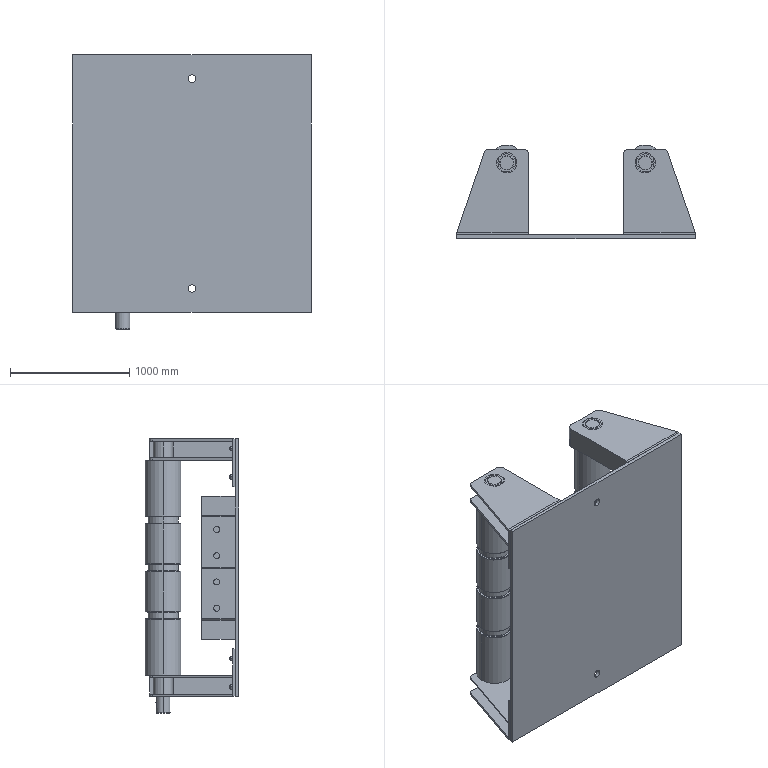Part | SolidWorks | features ReferencePattern 23, MirrorCompFeat 5, LocalLPattern 1 | 67 solids | 769 faces | box 2000 x 785 x 2300 mm | volume 484655330 mm3 | plane 380 | cylinder 260 | cone 81 | torus 48 | commonest cylinder face diameters 20 x64 22 x32 50 x32 170 x24 21 x16 36 x16